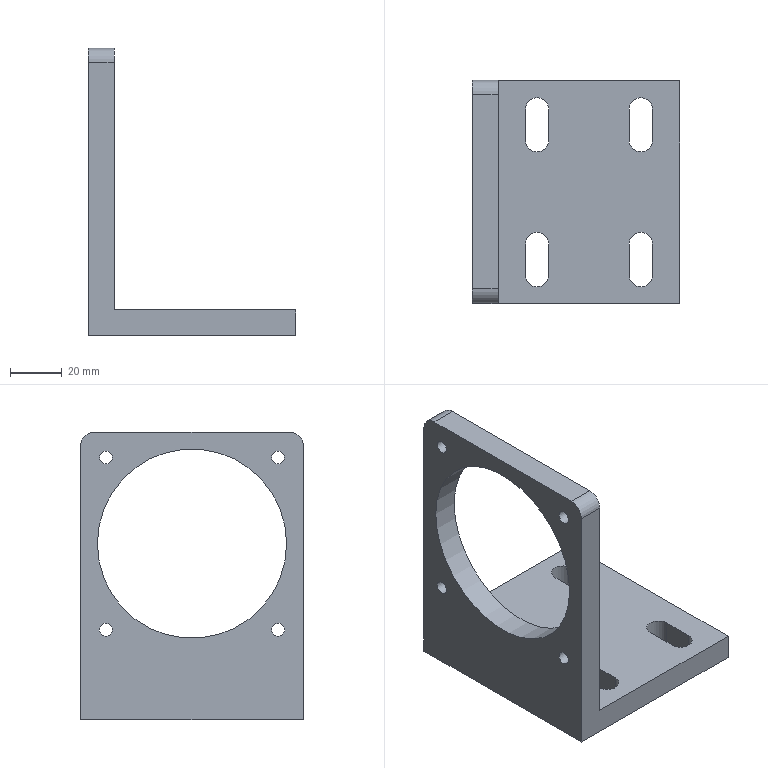Part | NX | features 5003_219_Bracket 2 | 1 solid | 31 faces | box 80 x 86 x 111 mm | volume 106026 mm3 | plane 16 | cylinder 15 | commonest cylinder face diameters 9 x8 5 x4 11 x2 73 x1
STEP:
#1=CARTESIAN_POINT('',(-21.725,90.734,-85.766));
#2=VERTEX_POINT('',#1);
#3=CARTESIAN_POINT('',(-21.725,88.234,-85.766));
#4=DIRECTION('',(-1.,0.,0.));
#5=DIRECTION('',(0.,1.,0.));
#6=AXIS2_PLACEMENT_3D('',#3,#4,#5);
#7=CIRCLE('',#6,2.5);
#8=EDGE_CURVE('',#2,#2,#7,.T.);
#9=ORIENTED_EDGE('',*,*,#8,.F.);
#10=EDGE_LOOP('',(#9));
#11=FACE_BOUND('',#10,.T.);
#12=CARTESIAN_POINT('',(-21.725,90.734,-152.234));
#13=VERTEX_POINT('',#12);
#14=CARTESIAN_POINT('',(-21.725,88.234,-152.234));
#15=DIRECTION('',(-1.,0.,0.));
#16=DIRECTION('',(0.,1.,0.));
#17=AXIS2_PLACEMENT_3D('',#14,#15,#16);
#18=CIRCLE('',#17,2.5);
#19=EDGE_CURVE('',#13,#13,#18,.T.);
#20=ORIENTED_EDGE('',*,*,#19,.F.);
#21=EDGE_LOOP('',(#20));
#22=FACE_BOUND('',#21,.T.);
#23=CARTESIAN_POINT('',(-21.725,24.266,-152.234));
#24=VERTEX_POINT('',#23);
#25=CARTESIAN_POINT('',(-21.725,21.766,-152.234));
#26=DIRECTION('',(-1.,0.,0.));
#27=DIRECTION('',(0.,1.,0.));
#28=AXIS2_PLACEMENT_3D('',#25,#26,#27);
#29=CIRCLE('',#28,2.5);
#30=EDGE_CURVE('',#24,#24,#29,.T.);
#31=ORIENTED_EDGE('',*,*,#30,.F.);
#32=EDGE_LOOP('',(#31));
#33=FACE_BOUND('',#32,.T.);
#34=CARTESIAN_POINT('',(-21.725,24.266,-85.766));
#35=VERTEX_POINT('',#34);
#36=CARTESIAN_POINT('',(-21.725,21.766,-85.766));
#37=DIRECTION('',(-1.,0.,0.));
#38=DIRECTION('',(0.,1.,0.));
#39=AXIS2_PLACEMENT_3D('',#36,#37,#38);
#40=CIRCLE('',#39,2.5);
#41=EDGE_CURVE('',#35,#35,#40,.T.);
#42=ORIENTED_EDGE('',*,*,#41,.F.);
#43=EDGE_LOOP('',(#42));
#44=FACE_BOUND('',#43,.T.);
#45=CARTESIAN_POINT('',(-21.725,91.5,-119.));
#46=VERTEX_POINT('',#45);
#47=CARTESIAN_POINT('',(-21.725,55.,-119.));
#48=DIRECTION('',(-1.,0.,0.));
#49=DIRECTION('',(0.,1.,0.));
#50=AXIS2_PLACEMENT_3D('',#47,#48,#49);
#51=CIRCLE('',#50,36.5);
#52=EDGE_CURVE('',#46,#46,#51,.T.);
#53=ORIENTED_EDGE('',*,*,#52,.F.);
#54=EDGE_LOOP('',(#53));
#55=FACE_BOUND('',#54,.T.);
#56=CARTESIAN_POINT('',(-21.725,12.,-187.));
#57=VERTEX_POINT('',#56);
#58=CARTESIAN_POINT('',(-21.725,12.,-81.5));
#59=VERTEX_POINT('',#58);
#60=CARTESIAN_POINT('',(-21.725,12.,-187.));
#61=DIRECTION('',(0.,0.,1.));
#62=VECTOR('',#61,1000.);
#63=LINE('',#60,#62);
#64=EDGE_CURVE('',#57,#59,#63,.T.);
#65=ORIENTED_EDGE('',*,*,#64,.T.);
#66=CARTESIAN_POINT('',(-21.725,17.5,-76.));
#67=VERTEX_POINT('',#66);
#68=CARTESIAN_POINT('',(-21.725,17.5,-81.5));
#69=DIRECTION('',(-1.,0.,0.));
#70=DIRECTION('',(0.,0.,1.));
#71=AXIS2_PLACEMENT_3D('',#68,#69,#70);
#72=CIRCLE('',#71,5.5);
#73=EDGE_CURVE('',#59,#67,#72,.T.);
#74=ORIENTED_EDGE('',*,*,#73,.T.);
#75=CARTESIAN_POINT('',(-21.725,92.5,-76.));
#76=VERTEX_POINT('',#75);
#77=CARTESIAN_POINT('',(-21.725,12.,-76.));
#78=DIRECTION('',(0.,1.,0.));
#79=VECTOR('',#78,1000.);
#80=LINE('',#77,#79);
#81=EDGE_CURVE('',#67,#76,#80,.T.);
#82=ORIENTED_EDGE('',*,*,#81,.T.);
#83=CARTESIAN_POINT('',(-21.725,98.,-81.5));
#84=VERTEX_POINT('',#83);
#85=CARTESIAN_POINT('',(-21.725,92.5,-81.5));
#86=DIRECTION('',(-1.,0.,0.));
#87=DIRECTION('',(0.,0.,1.));
#88=AXIS2_PLACEMENT_3D('',#85,#86,#87);
#89=CIRCLE('',#88,5.5);
#90=EDGE_CURVE('',#76,#84,#89,.T.);
#91=ORIENTED_EDGE('',*,*,#90,.T.);
#92=CARTESIAN_POINT('',(-21.725,98.,-187.));
#93=VERTEX_POINT('',#92);
#94=CARTESIAN_POINT('',(-21.725,98.,-187.));
#95=DIRECTION('',(0.,0.,1.));
#96=VECTOR('',#95,1000.);
#97=LINE('',#94,#96);
#98=EDGE_CURVE('',#93,#84,#97,.T.);
#99=ORIENTED_EDGE('',*,*,#98,.F.);
#100=CARTESIAN_POINT('',(-21.725,12.,-187.));
#101=DIRECTION('',(0.,1.,0.));
#102=VECTOR('',#101,1000.);
#103=LINE('',#100,#102);
#104=EDGE_CURVE('',#57,#93,#103,.T.);
#105=ORIENTED_EDGE('',*,*,#104,.F.);
#106=EDGE_LOOP('',(#65,#74,#82,#91,#99,#105));
#107=FACE_BOUND('',#106,.T.);
#108=CARTESIAN_POINT('',(-21.725,12.,-187.));
#109=DIRECTION('',(-1.,0.,0.));
#110=DIRECTION('',(0.,0.,1.));
#111=AXIS2_PLACEMENT_3D('',#108,#109,#110);
#112=PLANE('',#111);
#113=ADVANCED_FACE('',(#11,#22,#33,#44,#55,#107),#112,.T.);
#114=CARTESIAN_POINT('',(38.775,23.,-187.));
#115=VERTEX_POINT('',#114);
#116=CARTESIAN_POINT('',(47.775,23.,-187.));
#117=VERTEX_POINT('',#116);
#118=CARTESIAN_POINT('',(43.275,23.,-187.));
#119=DIRECTION('',(0.,0.,-1.));
#120=DIRECTION('',(-1.,0.,0.));
#121=AXIS2_PLACEMENT_3D('',#118,#119,#120);
#122=CIRCLE('',#121,4.5);
#123=EDGE_CURVE('',#115,#117,#122,.F.);
#124=ORIENTED_EDGE('',*,*,#123,.T.);
#125=CARTESIAN_POINT('',(47.775,35.,-187.));
#126=VERTEX_POINT('',#125);
#127=CARTESIAN_POINT('',(47.775,23.,-187.));
#128=DIRECTION('',(0.,1.,0.));
#129=VECTOR('',#128,1000.);
#130=LINE('',#127,#129);
#131=EDGE_CURVE('',#117,#126,#130,.T.);
#132=ORIENTED_EDGE('',*,*,#131,.T.);
#133=CARTESIAN_POINT('',(38.775,35.,-187.));
#134=VERTEX_POINT('',#133);
#135=CARTESIAN_POINT('',(43.275,35.,-187.));
#136=DIRECTION('',(0.,0.,-1.));
#137=DIRECTION('',(-1.,0.,0.));
#138=AXIS2_PLACEMENT_3D('',#135,#136,#137);
#139=CIRCLE('',#138,4.5);
#140=EDGE_CURVE('',#126,#134,#139,.F.);
#141=ORIENTED_EDGE('',*,*,#140,.T.);
#142=CARTESIAN_POINT('',(38.775,23.,-187.));
#143=DIRECTION('',(0.,-1.,0.));
#144=VECTOR('',#143,1000.);
#145=LINE('',#142,#144);
#146=EDGE_CURVE('',#134,#115,#145,.T.);
#147=ORIENTED_EDGE('',*,*,#146,.T.);
#148=EDGE_LOOP('',(#124,#132,#141,#147));
#149=FACE_BOUND('',#148,.T.);
#150=CARTESIAN_POINT('',(38.775,75.,-187.));
#151=VERTEX_POINT('',#150);
#152=CARTESIAN_POINT('',(47.775,75.,-187.));
#153=VERTEX_POINT('',#152);
#154=CARTESIAN_POINT('',(43.275,75.,-187.));
#155=DIRECTION('',(0.,0.,-1.));
#156=DIRECTION('',(-1.,0.,0.));
#157=AXIS2_PLACEMENT_3D('',#154,#155,#156);
#158=CIRCLE('',#157,4.5);
#159=EDGE_CURVE('',#151,#153,#158,.F.);
#160=ORIENTED_EDGE('',*,*,#159,.T.);
#161=CARTESIAN_POINT('',(47.775,87.,-187.));
#162=VERTEX_POINT('',#161);
#163=CARTESIAN_POINT('',(47.775,75.,-187.));
#164=DIRECTION('',(0.,1.,0.));
#165=VECTOR('',#164,1000.);
#166=LINE('',#163,#165);
#167=EDGE_CURVE('',#153,#162,#166,.T.);
#168=ORIENTED_EDGE('',*,*,#167,.T.);
#169=CARTESIAN_POINT('',(38.775,87.,-187.));
#170=VERTEX_POINT('',#169);
#171=CARTESIAN_POINT('',(43.275,87.,-187.));
#172=DIRECTION('',(0.,0.,-1.));
#173=DIRECTION('',(-1.,0.,0.));
#174=AXIS2_PLACEMENT_3D('',#171,#172,#173);
#175=CIRCLE('',#174,4.5);
#176=EDGE_CURVE('',#162,#170,#175,.F.);
#177=ORIENTED_EDGE('',*,*,#176,.T.);
#178=CARTESIAN_POINT('',(38.775,75.,-187.));
#179=DIRECTION('',(0.,-1.,0.));
#180=VECTOR('',#179,1000.);
#181=LINE('',#178,#180);
#182=EDGE_CURVE('',#170,#151,#181,.T.);
#183=ORIENTED_EDGE('',*,*,#182,.T.);
#184=EDGE_LOOP('',(#160,#168,#177,#183));
#185=FACE_BOUND('',#184,.T.);
#186=CARTESIAN_POINT('',(-1.225,75.,-187.));
#187=VERTEX_POINT('',#186);
#188=CARTESIAN_POINT('',(7.775,75.,-187.));
#189=VERTEX_POINT('',#188);
#190=CARTESIAN_POINT('',(3.275,75.,-187.));
#191=DIRECTION('',(0.,0.,-1.));
#192=DIRECTION('',(-1.,0.,0.));
#193=AXIS2_PLACEMENT_3D('',#190,#191,#192);
#194=CIRCLE('',#193,4.5);
#195=EDGE_CURVE('',#187,#189,#194,.F.);
#196=ORIENTED_EDGE('',*,*,#195,.T.);
#197=CARTESIAN_POINT('',(7.775,87.,-187.));
#198=VERTEX_POINT('',#197);
#199=CARTESIAN_POINT('',(7.775,75.,-187.));
#200=DIRECTION('',(0.,1.,0.));
#201=VECTOR('',#200,1000.);
#202=LINE('',#199,#201);
#203=EDGE_CURVE('',#189,#198,#202,.T.);
#204=ORIENTED_EDGE('',*,*,#203,.T.);
#205=CARTESIAN_POINT('',(-1.225,87.,-187.));
#206=VERTEX_POINT('',#205);
#207=CARTESIAN_POINT('',(3.275,87.,-187.));
#208=DIRECTION('',(0.,0.,-1.));
#209=DIRECTION('',(-1.,0.,0.));
#210=AXIS2_PLACEMENT_3D('',#207,#208,#209);
#211=CIRCLE('',#210,4.5);
#212=EDGE_CURVE('',#198,#206,#211,.F.);
#213=ORIENTED_EDGE('',*,*,#212,.T.);
#214=CARTESIAN_POINT('',(-1.225,75.,-187.));
#215=DIRECTION('',(0.,-1.,0.));
#216=VECTOR('',#215,1000.);
#217=LINE('',#214,#216);
#218=EDGE_CURVE('',#206,#187,#217,.T.);
#219=ORIENTED_EDGE('',*,*,#218,.T.);
#220=EDGE_LOOP('',(#196,#204,#213,#219));
#221=FACE_BOUND('',#220,.T.);
#222=CARTESIAN_POINT('',(-1.225,23.,-187.));
#223=VERTEX_POINT('',#222);
#224=CARTESIAN_POINT('',(7.775,23.,-187.));
#225=VERTEX_POINT('',#224);
#226=CARTESIAN_POINT('',(3.275,23.,-187.));
#227=DIRECTION('',(0.,0.,-1.));
#228=DIRECTION('',(-1.,0.,0.));
#229=AXIS2_PLACEMENT_3D('',#226,#227,#228);
#230=CIRCLE('',#229,4.5);
#231=EDGE_CURVE('',#223,#225,#230,.F.);
#232=ORIENTED_EDGE('',*,*,#231,.T.);
#233=CARTESIAN_POINT('',(7.775,35.,-187.));
#234=VERTEX_POINT('',#233);
#235=CARTESIAN_POINT('',(7.775,23.,-187.));
#236=DIRECTION('',(0.,1.,0.));
#237=VECTOR('',#236,1000.);
#238=LINE('',#235,#237);
#239=EDGE_CURVE('',#225,#234,#238,.T.);
#240=ORIENTED_EDGE('',*,*,#239,.T.);
#241=CARTESIAN_POINT('',(-1.225,35.,-187.));
#242=VERTEX_POINT('',#241);
#243=CARTESIAN_POINT('',(3.275,35.,-187.));
#244=DIRECTION('',(0.,0.,-1.));
#245=DIRECTION('',(-1.,0.,0.));
#246=AXIS2_PLACEMENT_3D('',#243,#244,#245);
#247=CIRCLE('',#246,4.5);
#248=EDGE_CURVE('',#234,#242,#247,.F.);
#249=ORIENTED_EDGE('',*,*,#248,.T.);
#250=CARTESIAN_POINT('',(-1.225,23.,-187.));
#251=DIRECTION('',(0.,-1.,0.));
#252=VECTOR('',#251,1000.);
#253=LINE('',#250,#252);
#254=EDGE_CURVE('',#242,#223,#253,.T.);
#255=ORIENTED_EDGE('',*,*,#254,.T.);
#256=EDGE_LOOP('',(#232,#240,#249,#255));
#257=FACE_BOUND('',#256,.T.);
#258=ORIENTED_EDGE('',*,*,#104,.T.);
#259=CARTESIAN_POINT('',(58.275,98.,-187.));
#260=VERTEX_POINT('',#259);
#261=CARTESIAN_POINT('',(-21.725,98.,-187.));
#262=DIRECTION('',(-1.,0.,0.));
#263=VECTOR('',#262,1000.);
#264=LINE('',#261,#263);
#265=EDGE_CURVE('',#260,#93,#264,.T.);
#266=ORIENTED_EDGE('',*,*,#265,.F.);
#267=CARTESIAN_POINT('',(58.275,12.,-187.));
#268=VERTEX_POINT('',#267);
#269=CARTESIAN_POINT('',(58.275,12.,-187.));
#270=DIRECTION('',(0.,1.,0.));
#271=VECTOR('',#270,1000.);
#272=LINE('',#269,#271);
#273=EDGE_CURVE('',#268,#260,#272,.T.);
#274=ORIENTED_EDGE('',*,*,#273,.F.);
#275=CARTESIAN_POINT('',(-21.725,12.,-187.));
#276=DIRECTION('',(-1.,0.,0.));
#277=VECTOR('',#276,1000.);
#278=LINE('',#275,#277);
#279=EDGE_CURVE('',#268,#57,#278,.T.);
#280=ORIENTED_EDGE('',*,*,#279,.T.);
#281=EDGE_LOOP('',(#258,#266,#274,#280));
#282=FACE_BOUND('',#281,.T.);
#283=CARTESIAN_POINT('',(-21.725,12.,-187.));
#284=DIRECTION('',(0.,0.,-1.));
#285=DIRECTION('',(-1.,0.,0.));
#286=AXIS2_PLACEMENT_3D('',#283,#284,#285);
#287=PLANE('',#286);
#288=ADVANCED_FACE('',(#149,#185,#221,#257,#282),#287,.T.);
#289=ORIENTED_EDGE('',*,*,#273,.T.);
#290=CARTESIAN_POINT('',(58.275,98.,-177.));
#291=VERTEX_POINT('',#290);
#292=CARTESIAN_POINT('',(58.275,98.,-187.));
#293=DIRECTION('',(0.,0.,-1.));
#294=VECTOR('',#293,1000.);
#295=LINE('',#292,#294);
#296=EDGE_CURVE('',#291,#260,#295,.T.);
#297=ORIENTED_EDGE('',*,*,#296,.F.);
#298=CARTESIAN_POINT('',(58.275,12.,-177.));
#299=VERTEX_POINT('',#298);
#300=CARTESIAN_POINT('',(58.275,12.,-177.));
#301=DIRECTION('',(0.,1.,0.));
#302=VECTOR('',#301,1000.);
#303=LINE('',#300,#302);
#304=EDGE_CURVE('',#299,#291,#303,.T.);
#305=ORIENTED_EDGE('',*,*,#304,.F.);
#306=CARTESIAN_POINT('',(58.275,12.,-187.));
#307=DIRECTION('',(0.,0.,-1.));
#308=VECTOR('',#307,1000.);
#309=LINE('',#306,#308);
#310=EDGE_CURVE('',#299,#268,#309,.T.);
#311=ORIENTED_EDGE('',*,*,#310,.T.);
#312=EDGE_LOOP('',(#289,#297,#305,#311));
#313=FACE_BOUND('',#312,.T.);
#314=CARTESIAN_POINT('',(58.275,12.,-187.));
#315=DIRECTION('',(1.,0.,0.));
#316=DIRECTION('',(0.,-1.,0.));
#317=AXIS2_PLACEMENT_3D('',#314,#315,#316);
#318=PLANE('',#317);
#319=ADVANCED_FACE('',(#313),#318,.T.);
#320=CARTESIAN_POINT('',(38.775,23.,-177.));
#321=VERTEX_POINT('',#320);
#322=CARTESIAN_POINT('',(47.775,23.,-177.));
#323=VERTEX_POINT('',#322);
#324=CARTESIAN_POINT('',(43.275,23.,-177.));
#325=DIRECTION('',(0.,0.,1.));
#326=DIRECTION('',(1.,0.,0.));
#327=AXIS2_PLACEMENT_3D('',#324,#325,#326);
#328=CIRCLE('',#327,4.5);
#329=EDGE_CURVE('',#321,#323,#328,.T.);
#330=ORIENTED_EDGE('',*,*,#329,.F.);
#331=CARTESIAN_POINT('',(38.775,35.,-177.));
#332=VERTEX_POINT('',#331);
#333=CARTESIAN_POINT('',(38.775,23.,-177.));
#334=DIRECTION('',(0.,-1.,0.));
#335=VECTOR('',#334,1000.);
#336=LINE('',#333,#335);
#337=EDGE_CURVE('',#332,#321,#336,.T.);
#338=ORIENTED_EDGE('',*,*,#337,.F.);
#339=CARTESIAN_POINT('',(47.775,35.,-177.));
#340=VERTEX_POINT('',#339);
#341=CARTESIAN_POINT('',(43.275,35.,-177.));
#342=DIRECTION('',(0.,0.,1.));
#343=DIRECTION('',(1.,0.,0.));
#344=AXIS2_PLACEMENT_3D('',#341,#342,#343);
#345=CIRCLE('',#344,4.5);
#346=EDGE_CURVE('',#340,#332,#345,.T.);
#347=ORIENTED_EDGE('',*,*,#346,.F.);
#348=CARTESIAN_POINT('',(47.775,23.,-177.));
#349=DIRECTION('',(0.,1.,0.));
#350=VECTOR('',#349,1000.);
#351=LINE('',#348,#350);
#352=EDGE_CURVE('',#323,#340,#351,.T.);
#353=ORIENTED_EDGE('',*,*,#352,.F.);
#354=EDGE_LOOP('',(#330,#338,#347,#353));
#355=FACE_BOUND('',#354,.T.);
#356=CARTESIAN_POINT('',(38.775,75.,-177.));
#357=VERTEX_POINT('',#356);
#358=CARTESIAN_POINT('',(47.775,75.,-177.));
#359=VERTEX_POINT('',#358);
#360=CARTESIAN_POINT('',(43.275,75.,-177.));
#361=DIRECTION('',(0.,0.,1.));
#362=DIRECTION('',(1.,0.,0.));
#363=AXIS2_PLACEMENT_3D('',#360,#361,#362);
#364=CIRCLE('',#363,4.5);
#365=EDGE_CURVE('',#357,#359,#364,.T.);
#366=ORIENTED_EDGE('',*,*,#365,.F.);
#367=CARTESIAN_POINT('',(38.775,87.,-177.));
#368=VERTEX_POINT('',#367);
#369=CARTESIAN_POINT('',(38.775,75.,-177.));
#370=DIRECTION('',(0.,-1.,0.));
#371=VECTOR('',#370,1000.);
#372=LINE('',#369,#371);
#373=EDGE_CURVE('',#368,#357,#372,.T.);
#374=ORIENTED_EDGE('',*,*,#373,.F.);
#375=CARTESIAN_POINT('',(47.775,87.,-177.));
#376=VERTEX_POINT('',#375);
#377=CARTESIAN_POINT('',(43.275,87.,-177.));
#378=DIRECTION('',(0.,0.,1.));
#379=DIRECTION('',(1.,0.,0.));
#380=AXIS2_PLACEMENT_3D('',#377,#378,#379);
#381=CIRCLE('',#380,4.5);
#382=EDGE_CURVE('',#376,#368,#381,.T.);
#383=ORIENTED_EDGE('',*,*,#382,.F.);
#384=CARTESIAN_POINT('',(47.775,75.,-177.));
#385=DIRECTION('',(0.,1.,0.));
#386=VECTOR('',#385,1000.);
#387=LINE('',#384,#386);
#388=EDGE_CURVE('',#359,#376,#387,.T.);
#389=ORIENTED_EDGE('',*,*,#388,.F.);
#390=EDGE_LOOP('',(#366,#374,#383,#389));
#391=FACE_BOUND('',#390,.T.);
#392=CARTESIAN_POINT('',(-1.225,75.,-177.));
#393=VERTEX_POINT('',#392);
#394=CARTESIAN_POINT('',(7.775,75.,-177.));
#395=VERTEX_POINT('',#394);
#396=CARTESIAN_POINT('',(3.275,75.,-177.));
#397=DIRECTION('',(0.,0.,1.));
#398=DIRECTION('',(1.,0.,0.));
#399=AXIS2_PLACEMENT_3D('',#396,#397,#398);
#400=CIRCLE('',#399,4.5);
#401=EDGE_CURVE('',#393,#395,#400,.T.);
#402=ORIENTED_EDGE('',*,*,#401,.F.);
#403=CARTESIAN_POINT('',(-1.225,87.,-177.));
#404=VERTEX_POINT('',#403);
#405=CARTESIAN_POINT('',(-1.225,75.,-177.));
#406=DIRECTION('',(0.,-1.,0.));
#407=VECTOR('',#406,1000.);
#408=LINE('',#405,#407);
#409=EDGE_CURVE('',#404,#393,#408,.T.);
#410=ORIENTED_EDGE('',*,*,#409,.F.);
#411=CARTESIAN_POINT('',(7.775,87.,-177.));
#412=VERTEX_POINT('',#411);
#413=CARTESIAN_POINT('',(3.275,87.,-177.));
#414=DIRECTION('',(0.,0.,1.));
#415=DIRECTION('',(1.,0.,0.));
#416=AXIS2_PLACEMENT_3D('',#413,#414,#415);
#417=CIRCLE('',#416,4.5);
#418=EDGE_CURVE('',#412,#404,#417,.T.);
#419=ORIENTED_EDGE('',*,*,#418,.F.);
#420=CARTESIAN_POINT('',(7.775,75.,-177.));
#421=DIRECTION('',(0.,1.,0.));
#422=VECTOR('',#421,1000.);
#423=LINE('',#420,#422);
#424=EDGE_CURVE('',#395,#412,#423,.T.);
#425=ORIENTED_EDGE('',*,*,#424,.F.);
#426=EDGE_LOOP('',(#402,#410,#419,#425));
#427=FACE_BOUND('',#426,.T.);
#428=CARTESIAN_POINT('',(-1.225,23.,-177.));
#429=VERTEX_POINT('',#428);
#430=CARTESIAN_POINT('',(7.775,23.,-177.));
#431=VERTEX_POINT('',#430);
#432=CARTESIAN_POINT('',(3.275,23.,-177.));
#433=DIRECTION('',(0.,0.,1.));
#434=DIRECTION('',(1.,0.,0.));
#435=AXIS2_PLACEMENT_3D('',#432,#433,#434);
#436=CIRCLE('',#435,4.5);
#437=EDGE_CURVE('',#429,#431,#436,.T.);
#438=ORIENTED_EDGE('',*,*,#437,.F.);
#439=CARTESIAN_POINT('',(-1.225,35.,-177.));
#440=VERTEX_POINT('',#439);
#441=CARTESIAN_POINT('',(-1.225,23.,-177.));
#442=DIRECTION('',(0.,-1.,0.));
#443=VECTOR('',#442,1000.);
#444=LINE('',#441,#443);
#445=EDGE_CURVE('',#440,#429,#444,.T.);
#446=ORIENTED_EDGE('',*,*,#445,.F.);
#447=CARTESIAN_POINT('',(7.775,35.,-177.));
#448=VERTEX_POINT('',#447);
#449=CARTESIAN_POINT('',(3.275,35.,-177.));
#450=DIRECTION('',(0.,0.,1.));
#451=DIRECTION('',(1.,0.,0.));
#452=AXIS2_PLACEMENT_3D('',#449,#450,#451);
#453=CIRCLE('',#452,4.5);
#454=EDGE_CURVE('',#448,#440,#453,.T.);
#455=ORIENTED_EDGE('',*,*,#454,.F.);
#456=CARTESIAN_POINT('',(7.775,23.,-177.));
#457=DIRECTION('',(0.,1.,0.));
#458=VECTOR('',#457,1000.);
#459=LINE('',#456,#458);
#460=EDGE_CURVE('',#431,#448,#459,.T.);
#461=ORIENTED_EDGE('',*,*,#460,.F.);
#462=EDGE_LOOP('',(#438,#446,#455,#461));
#463=FACE_BOUND('',#462,.T.);
#464=ORIENTED_EDGE('',*,*,#304,.T.);
#465=CARTESIAN_POINT('',(-11.725,98.,-177.));
#466=VERTEX_POINT('',#465);
#467=CARTESIAN_POINT('',(-11.725,98.,-177.));
#468=DIRECTION('',(1.,0.,0.));
#469=VECTOR('',#468,1000.);
#470=LINE('',#467,#469);
#471=EDGE_CURVE('',#466,#291,#470,.T.);
#472=ORIENTED_EDGE('',*,*,#471,.F.);
#473=CARTESIAN_POINT('',(-11.725,12.,-177.));
#474=VERTEX_POINT('',#473);
#475=CARTESIAN_POINT('',(-11.725,12.,-177.));
#476=DIRECTION('',(0.,1.,0.));
#477=VECTOR('',#476,1000.);
#478=LINE('',#475,#477);
#479=EDGE_CURVE('',#474,#466,#478,.T.);
#480=ORIENTED_EDGE('',*,*,#479,.F.);
#481=CARTESIAN_POINT('',(-11.725,12.,-177.));
#482=DIRECTION('',(1.,0.,0.));
#483=VECTOR('',#482,1000.);
#484=LINE('',#481,#483);
#485=EDGE_CURVE('',#474,#299,#484,.T.);
#486=ORIENTED_EDGE('',*,*,#485,.T.);
#487=EDGE_LOOP('',(#464,#472,#480,#486));
#488=FACE_BOUND('',#487,.T.);
#489=CARTESIAN_POINT('',(-11.725,12.,-177.));
#490=DIRECTION('',(0.,0.,1.));
#491=DIRECTION('',(1.,0.,0.));
#492=AXIS2_PLACEMENT_3D('',#489,#490,#491);
#493=PLANE('',#492);
#494=ADVANCED_FACE('',(#355,#391,#427,#463,#488),#493,.T.);
#495=CARTESIAN_POINT('',(-11.725,85.734,-85.766));
#496=VERTEX_POINT('',#495);
#497=CARTESIAN_POINT('',(-11.725,88.234,-85.766));
#498=DIRECTION('',(1.,0.,0.));
#499=DIRECTION('',(0.,-1.,0.));
#500=AXIS2_PLACEMENT_3D('',#497,#498,#499);
#501=CIRCLE('',#500,2.5);
#502=EDGE_CURVE('',#496,#496,#501,.T.);
#503=ORIENTED_EDGE('',*,*,#502,.F.);
#504=EDGE_LOOP('',(#503));
#505=FACE_BOUND('',#504,.T.);
#506=CARTESIAN_POINT('',(-11.725,85.734,-152.234));
#507=VERTEX_POINT('',#506);
#508=CARTESIAN_POINT('',(-11.725,88.234,-152.234));
#509=DIRECTION('',(1.,0.,0.));
#510=DIRECTION('',(0.,-1.,0.));
#511=AXIS2_PLACEMENT_3D('',#508,#509,#510);
#512=CIRCLE('',#511,2.5);
#513=EDGE_CURVE('',#507,#507,#512,.T.);
#514=ORIENTED_EDGE('',*,*,#513,.F.);
#515=EDGE_LOOP('',(#514));
#516=FACE_BOUND('',#515,.T.);
#517=CARTESIAN_POINT('',(-11.725,19.266,-152.234));
#518=VERTEX_POINT('',#517);
#519=CARTESIAN_POINT('',(-11.725,21.766,-152.234));
#520=DIRECTION('',(1.,0.,0.));
#521=DIRECTION('',(0.,-1.,0.));
#522=AXIS2_PLACEMENT_3D('',#519,#520,#521);
#523=CIRCLE('',#522,2.5);
#524=EDGE_CURVE('',#518,#518,#523,.T.);
#525=ORIENTED_EDGE('',*,*,#524,.F.);
#526=EDGE_LOOP('',(#525));
#527=FACE_BOUND('',#526,.T.);
#528=CARTESIAN_POINT('',(-11.725,19.266,-85.766));
#529=VERTEX_POINT('',#528);
#530=CARTESIAN_POINT('',(-11.725,21.766,-85.766));
#531=DIRECTION('',(1.,0.,0.));
#532=DIRECTION('',(0.,-1.,0.));
#533=AXIS2_PLACEMENT_3D('',#530,#531,#532);
#534=CIRCLE('',#533,2.5);
#535=EDGE_CURVE('',#529,#529,#534,.T.);
#536=ORIENTED_EDGE('',*,*,#535,.F.);
#537=EDGE_LOOP('',(#536));
#538=FACE_BOUND('',#537,.T.);
#539=CARTESIAN_POINT('',(-11.725,18.5,-119.));
#540=VERTEX_POINT('',#539);
#541=CARTESIAN_POINT('',(-11.725,55.,-119.));
#542=DIRECTION('',(1.,0.,0.));
#543=DIRECTION('',(0.,-1.,0.));
#544=AXIS2_PLACEMENT_3D('',#541,#542,#543);
#545=CIRCLE('',#544,36.5);
#546=EDGE_CURVE('',#540,#540,#545,.F.);
#547=ORIENTED_EDGE('',*,*,#546,.T.);
#548=EDGE_LOOP('',(#547));
#549=FACE_BOUND('',#548,.T.);
#550=CARTESIAN_POINT('',(-11.725,17.5,-76.));
#551=VERTEX_POINT('',#550);
#552=CARTESIAN_POINT('',(-11.725,92.5,-76.));
#553=VERTEX_POINT('',#552);
#554=CARTESIAN_POINT('',(-11.725,12.,-76.));
#555=DIRECTION('',(0.,1.,0.));
#556=VECTOR('',#555,1000.);
#557=LINE('',#554,#556);
#558=EDGE_CURVE('',#551,#553,#557,.T.);
#559=ORIENTED_EDGE('',*,*,#558,.F.);
#560=CARTESIAN_POINT('',(-11.725,12.,-81.5));
#561=VERTEX_POINT('',#560);
#562=CARTESIAN_POINT('',(-11.725,17.5,-81.5));
#563=DIRECTION('',(1.,0.,0.));
#564=DIRECTION('',(0.,-1.,0.));
#565=AXIS2_PLACEMENT_3D('',#562,#563,#564);
#566=CIRCLE('',#565,5.5);
#567=EDGE_CURVE('',#551,#561,#566,.T.);
#568=ORIENTED_EDGE('',*,*,#567,.T.);
#569=CARTESIAN_POINT('',(-11.725,12.,-177.));
#570=DIRECTION('',(0.,0.,-1.));
#571=VECTOR('',#570,1000.);
#572=LINE('',#569,#571);
#573=EDGE_CURVE('',#561,#474,#572,.T.);
#574=ORIENTED_EDGE('',*,*,#573,.T.);
#575=ORIENTED_EDGE('',*,*,#479,.T.);
#576=CARTESIAN_POINT('',(-11.725,98.,-81.5));
#577=VERTEX_POINT('',#576);
#578=CARTESIAN_POINT('',(-11.725,98.,-177.));
#579=DIRECTION('',(0.,0.,-1.));
#580=VECTOR('',#579,1000.);
#581=LINE('',#578,#580);
#582=EDGE_CURVE('',#577,#466,#581,.T.);
#583=ORIENTED_EDGE('',*,*,#582,.F.);
#584=CARTESIAN_POINT('',(-11.725,92.5,-81.5));
#585=DIRECTION('',(1.,0.,0.));
#586=DIRECTION('',(0.,-1.,0.));
#587=AXIS2_PLACEMENT_3D('',#584,#585,#586);
#588=CIRCLE('',#587,5.5);
#589=EDGE_CURVE('',#577,#553,#588,.T.);
#590=ORIENTED_EDGE('',*,*,#589,.T.);
#591=EDGE_LOOP('',(#559,#568,#574,#575,#583,#590));
#592=FACE_BOUND('',#591,.T.);
#593=CARTESIAN_POINT('',(-11.725,12.,-177.));
#594=DIRECTION('',(1.,0.,0.));
#595=DIRECTION('',(0.,-1.,0.));
#596=AXIS2_PLACEMENT_3D('',#593,#594,#595);
#597=PLANE('',#596);
#598=ADVANCED_FACE('',(#505,#516,#527,#538,#549,#592),#597,.T.);
#599=ORIENTED_EDGE('',*,*,#81,.F.);
#600=CARTESIAN_POINT('',(-11.725,17.5,-76.));
#601=DIRECTION('',(1.,0.,0.));
#602=VECTOR('',#601,1000.);
#603=LINE('',#600,#602);
#604=EDGE_CURVE('',#67,#551,#603,.T.);
#605=ORIENTED_EDGE('',*,*,#604,.T.);
#606=ORIENTED_EDGE('',*,*,#558,.T.);
#607=CARTESIAN_POINT('',(-21.725,92.5,-76.));
#608=DIRECTION('',(1.,0.,0.));
#609=VECTOR('',#608,1000.);
#610=LINE('',#607,#609);
#611=EDGE_CURVE('',#553,#76,#610,.F.);
#612=ORIENTED_EDGE('',*,*,#611,.T.);
#613=EDGE_LOOP('',(#599,#605,#606,#612));
#614=FACE_BOUND('',#613,.T.);
#615=CARTESIAN_POINT('',(-21.725,12.,-76.));
#616=DIRECTION('',(0.,0.,1.));
#617=DIRECTION('',(1.,0.,0.));
#618=AXIS2_PLACEMENT_3D('',#615,#616,#617);
#619=PLANE('',#618);
#620=ADVANCED_FACE('',(#614),#619,.T.);
#621=ORIENTED_EDGE('',*,*,#573,.F.);
#622=CARTESIAN_POINT('',(-21.725,12.,-81.5));
#623=DIRECTION('',(1.,0.,0.));
#624=VECTOR('',#623,1000.);
#625=LINE('',#622,#624);
#626=EDGE_CURVE('',#561,#59,#625,.F.);
#627=ORIENTED_EDGE('',*,*,#626,.T.);
#628=ORIENTED_EDGE('',*,*,#64,.F.);
#629=ORIENTED_EDGE('',*,*,#279,.F.);
#630=ORIENTED_EDGE('',*,*,#310,.F.);
#631=ORIENTED_EDGE('',*,*,#485,.F.);
#632=EDGE_LOOP('',(#621,#627,#628,#629,#630,#631));
#633=FACE_BOUND('',#632,.T.);
#634=CARTESIAN_POINT('',(-21.725,12.,-187.));
#635=DIRECTION('',(0.,1.,0.));
#636=DIRECTION('',(1.,0.,0.));
#637=AXIS2_PLACEMENT_3D('',#634,#635,#636);
#638=PLANE('',#637);
#639=ADVANCED_FACE('',(#633),#638,.F.);
#640=ORIENTED_EDGE('',*,*,#98,.T.);
#641=CARTESIAN_POINT('',(-21.725,98.,-81.5));
#642=DIRECTION('',(1.,0.,0.));
#643=VECTOR('',#642,1000.);
#644=LINE('',#641,#643);
#645=EDGE_CURVE('',#84,#577,#644,.T.);
#646=ORIENTED_EDGE('',*,*,#645,.T.);
#647=ORIENTED_EDGE('',*,*,#582,.T.);
#648=ORIENTED_EDGE('',*,*,#471,.T.);
#649=ORIENTED_EDGE('',*,*,#296,.T.);
#650=ORIENTED_EDGE('',*,*,#265,.T.);
#651=EDGE_LOOP('',(#640,#646,#647,#648,#649,#650));
#652=FACE_BOUND('',#651,.T.);
#653=CARTESIAN_POINT('',(-21.725,98.,-187.));
#654=DIRECTION('',(0.,1.,0.));
#655=DIRECTION('',(1.,0.,0.));
#656=AXIS2_PLACEMENT_3D('',#653,#654,#655);
#657=PLANE('',#656);
#658=ADVANCED_FACE('',(#652),#657,.T.);
#659=ORIENTED_EDGE('',*,*,#546,.F.);
#660=EDGE_LOOP('',(#659));
#661=FACE_BOUND('',#660,.T.);
#662=ORIENTED_EDGE('',*,*,#52,.T.);
#663=EDGE_LOOP('',(#662));
#664=FACE_BOUND('',#663,.T.);
#665=CARTESIAN_POINT('',(58.276,55.,-119.));
#666=DIRECTION('',(-1.,0.,0.));
#667=DIRECTION('',(0.,1.,0.));
#668=AXIS2_PLACEMENT_3D('',#665,#666,#667);
#669=CYLINDRICAL_SURFACE('',#668,36.5);
#670=ADVANCED_FACE('',(#661,#664),#669,.F.);
#671=CARTESIAN_POINT('',(-1.225,23.,-187.001));
#672=DIRECTION('',(0.,0.,1.));
#673=VECTOR('',#672,1000.);
#674=LINE('',#671,#673);
#675=EDGE_CURVE('',#223,#429,#674,.T.);
#676=ORIENTED_EDGE('',*,*,#675,.T.);
#677=ORIENTED_EDGE('',*,*,#437,.T.);
#678=CARTESIAN_POINT('',(7.775,23.,-187.001));
#679=DIRECTION('',(0.,0.,1.));
#680=VECTOR('',#679,1000.);
#681=LINE('',#678,#680);
#682=EDGE_CURVE('',#225,#431,#681,.T.);
#683=ORIENTED_EDGE('',*,*,#682,.F.);
#684=ORIENTED_EDGE('',*,*,#231,.F.);
#685=EDGE_LOOP('',(#676,#677,#683,#684));
#686=FACE_BOUND('',#685,.T.);
#687=CARTESIAN_POINT('',(3.275,23.,-187.001));
#688=DIRECTION('',(0.,0.,1.));
#689=DIRECTION('',(1.,0.,0.));
#690=AXIS2_PLACEMENT_3D('',#687,#688,#689);
#691=CYLINDRICAL_SURFACE('',#690,4.5);
#692=ADVANCED_FACE('',(#686),#691,.F.);
#693=CARTESIAN_POINT('',(-1.225,35.,-187.001));
#694=DIRECTION('',(0.,0.,1.));
#695=VECTOR('',#694,1000.);
#696=LINE('',#693,#695);
#697=EDGE_CURVE('',#242,#440,#696,.T.);
#698=ORIENTED_EDGE('',*,*,#697,.T.);
#699=ORIENTED_EDGE('',*,*,#445,.T.);
#700=ORIENTED_EDGE('',*,*,#675,.F.);
#701=ORIENTED_EDGE('',*,*,#254,.F.);
#702=EDGE_LOOP('',(#698,#699,#700,#701));
#703=FACE_BOUND('',#702,.T.);
#704=CARTESIAN_POINT('',(-1.225,23.,-187.001));
#705=DIRECTION('',(-1.,0.,0.));
#706=DIRECTION('',(0.,1.,0.));
#707=AXIS2_PLACEMENT_3D('',#704,#705,#706);
#708=PLANE('',#707);
#709=ADVANCED_FACE('',(#703),#708,.F.);
#710=CARTESIAN_POINT('',(7.775,35.,-187.001));
#711=DIRECTION('',(0.,0.,1.));
#712=VECTOR('',#711,1000.);
#713=LINE('',#710,#712);
#714=EDGE_CURVE('',#234,#448,#713,.T.);
#715=ORIENTED_EDGE('',*,*,#714,.T.);
#716=ORIENTED_EDGE('',*,*,#454,.T.);
#717=ORIENTED_EDGE('',*,*,#697,.F.);
#718=ORIENTED_EDGE('',*,*,#248,.F.);
#719=EDGE_LOOP('',(#715,#716,#717,#718));
#720=FACE_BOUND('',#719,.T.);
#721=CARTESIAN_POINT('',(3.275,35.,-187.001));
#722=DIRECTION('',(0.,0.,1.));
#723=DIRECTION('',(1.,0.,0.));
#724=AXIS2_PLACEMENT_3D('',#721,#722,#723);
#725=CYLINDRICAL_SURFACE('',#724,4.5);
#726=ADVANCED_FACE('',(#720),#725,.F.);
#727=ORIENTED_EDGE('',*,*,#682,.T.);
#728=ORIENTED_EDGE('',*,*,#460,.T.);
#729=ORIENTED_EDGE('',*,*,#714,.F.);
#730=ORIENTED_EDGE('',*,*,#239,.F.);
#731=EDGE_LOOP('',(#727,#728,#729,#730));
#732=FACE_BOUND('',#731,.T.);
#733=CARTESIAN_POINT('',(7.775,23.,-187.001));
#734=DIRECTION('',(1.,0.,0.));
#735=DIRECTION('',(0.,-1.,0.));
#736=AXIS2_PLACEMENT_3D('',#733,#734,#735);
#737=PLANE('',#736);
#738=ADVANCED_FACE('',(#732),#737,.F.);
#739=CARTESIAN_POINT('',(-1.225,75.,-187.001));
#740=DIRECTION('',(0.,0.,1.));
#741=VECTOR('',#740,1000.);
#742=LINE('',#739,#741);
#743=EDGE_CURVE('',#187,#393,#742,.T.);
#744=ORIENTED_EDGE('',*,*,#743,.T.);
#745=ORIENTED_EDGE('',*,*,#401,.T.);
#746=CARTESIAN_POINT('',(7.775,75.,-187.001));
#747=DIRECTION('',(0.,0.,1.));
#748=VECTOR('',#747,1000.);
#749=LINE('',#746,#748);
#750=EDGE_CURVE('',#189,#395,#749,.T.);
#751=ORIENTED_EDGE('',*,*,#750,.F.);
#752=ORIENTED_EDGE('',*,*,#195,.F.);
#753=EDGE_LOOP('',(#744,#745,#751,#752));
#754=FACE_BOUND('',#753,.T.);
#755=CARTESIAN_POINT('',(3.275,75.,-187.001));
#756=DIRECTION('',(0.,0.,1.));
#757=DIRECTION('',(1.,0.,0.));
#758=AXIS2_PLACEMENT_3D('',#755,#756,#757);
#759=CYLINDRICAL_SURFACE('',#758,4.5);
#760=ADVANCED_FACE('',(#754),#759,.F.);
#761=CARTESIAN_POINT('',(-1.225,87.,-187.001));
#762=DIRECTION('',(0.,0.,1.));
#763=VECTOR('',#762,1000.);
#764=LINE('',#761,#763);
#765=EDGE_CURVE('',#206,#404,#764,.T.);
#766=ORIENTED_EDGE('',*,*,#765,.T.);
#767=ORIENTED_EDGE('',*,*,#409,.T.);
#768=ORIENTED_EDGE('',*,*,#743,.F.);
#769=ORIENTED_EDGE('',*,*,#218,.F.);
#770=EDGE_LOOP('',(#766,#767,#768,#769));
#771=FACE_BOUND('',#770,.T.);
#772=CARTESIAN_POINT('',(-1.225,75.,-187.001));
#773=DIRECTION('',(-1.,0.,0.));
#774=DIRECTION('',(0.,1.,0.));
#775=AXIS2_PLACEMENT_3D('',#772,#773,#774);
#776=PLANE('',#775);
#777=ADVANCED_FACE('',(#771),#776,.F.);
#778=CARTESIAN_POINT('',(7.775,87.,-187.001));
#779=DIRECTION('',(0.,0.,1.));
#780=VECTOR('',#779,1000.);
#781=LINE('',#778,#780);
#782=EDGE_CURVE('',#198,#412,#781,.T.);
#783=ORIENTED_EDGE('',*,*,#782,.T.);
#784=ORIENTED_EDGE('',*,*,#418,.T.);
#785=ORIENTED_EDGE('',*,*,#765,.F.);
#786=ORIENTED_EDGE('',*,*,#212,.F.);
#787=EDGE_LOOP('',(#783,#784,#785,#786));
#788=FACE_BOUND('',#787,.T.);
#789=CARTESIAN_POINT('',(3.275,87.,-187.001));
#790=DIRECTION('',(0.,0.,1.));
#791=DIRECTION('',(1.,0.,0.));
#792=AXIS2_PLACEMENT_3D('',#789,#790,#791);
#793=CYLINDRICAL_SURFACE('',#792,4.5);
#794=ADVANCED_FACE('',(#788),#793,.F.);
#795=ORIENTED_EDGE('',*,*,#750,.T.);
#796=ORIENTED_EDGE('',*,*,#424,.T.);
#797=ORIENTED_EDGE('',*,*,#782,.F.);
#798=ORIENTED_EDGE('',*,*,#203,.F.);
#799=EDGE_LOOP('',(#795,#796,#797,#798));
#800=FACE_BOUND('',#799,.T.);
#801=CARTESIAN_POINT('',(7.775,75.,-187.001));
#802=DIRECTION('',(1.,0.,0.));
#803=DIRECTION('',(0.,-1.,0.));
#804=AXIS2_PLACEMENT_3D('',#801,#802,#803);
#805=PLANE('',#804);
#806=ADVANCED_FACE('',(#800),#805,.F.);
#807=CARTESIAN_POINT('',(38.775,75.,-187.001));
#808=DIRECTION('',(0.,0.,1.));
#809=VECTOR('',#808,1000.);
#810=LINE('',#807,#809);
#811=EDGE_CURVE('',#151,#357,#810,.T.);
#812=ORIENTED_EDGE('',*,*,#811,.T.);
#813=ORIENTED_EDGE('',*,*,#365,.T.);
#814=CARTESIAN_POINT('',(47.775,75.,-187.001));
#815=DIRECTION('',(0.,0.,1.));
#816=VECTOR('',#815,1000.);
#817=LINE('',#814,#816);
#818=EDGE_CURVE('',#153,#359,#817,.T.);
#819=ORIENTED_EDGE('',*,*,#818,.F.);
#820=ORIENTED_EDGE('',*,*,#159,.F.);
#821=EDGE_LOOP('',(#812,#813,#819,#820));
#822=FACE_BOUND('',#821,.T.);
#823=CARTESIAN_POINT('',(43.275,75.,-187.001));
#824=DIRECTION('',(0.,0.,1.));
#825=DIRECTION('',(1.,0.,0.));
#826=AXIS2_PLACEMENT_3D('',#823,#824,#825);
#827=CYLINDRICAL_SURFACE('',#826,4.5);
#828=ADVANCED_FACE('',(#822),#827,.F.);
#829=CARTESIAN_POINT('',(38.775,87.,-187.001));
#830=DIRECTION('',(0.,0.,1.));
#831=VECTOR('',#830,1000.);
#832=LINE('',#829,#831);
#833=EDGE_CURVE('',#170,#368,#832,.T.);
#834=ORIENTED_EDGE('',*,*,#833,.T.);
#835=ORIENTED_EDGE('',*,*,#373,.T.);
#836=ORIENTED_EDGE('',*,*,#811,.F.);
#837=ORIENTED_EDGE('',*,*,#182,.F.);
#838=EDGE_LOOP('',(#834,#835,#836,#837));
#839=FACE_BOUND('',#838,.T.);
#840=CARTESIAN_POINT('',(38.775,75.,-187.001));
#841=DIRECTION('',(-1.,0.,0.));
#842=DIRECTION('',(0.,1.,0.));
#843=AXIS2_PLACEMENT_3D('',#840,#841,#842);
#844=PLANE('',#843);
#845=ADVANCED_FACE('',(#839),#844,.F.);
#846=CARTESIAN_POINT('',(47.775,87.,-187.001));
#847=DIRECTION('',(0.,0.,1.));
#848=VECTOR('',#847,1000.);
#849=LINE('',#846,#848);
#850=EDGE_CURVE('',#162,#376,#849,.T.);
#851=ORIENTED_EDGE('',*,*,#850,.T.);
#852=ORIENTED_EDGE('',*,*,#382,.T.);
#853=ORIENTED_EDGE('',*,*,#833,.F.);
#854=ORIENTED_EDGE('',*,*,#176,.F.);
#855=EDGE_LOOP('',(#851,#852,#853,#854));
#856=FACE_BOUND('',#855,.T.);
#857=CARTESIAN_POINT('',(43.275,87.,-187.001));
#858=DIRECTION('',(0.,0.,1.));
#859=DIRECTION('',(1.,0.,0.));
#860=AXIS2_PLACEMENT_3D('',#857,#858,#859);
#861=CYLINDRICAL_SURFACE('',#860,4.5);
#862=ADVANCED_FACE('',(#856),#861,.F.);
#863=ORIENTED_EDGE('',*,*,#818,.T.);
#864=ORIENTED_EDGE('',*,*,#388,.T.);
#865=ORIENTED_EDGE('',*,*,#850,.F.);
#866=ORIENTED_EDGE('',*,*,#167,.F.);
#867=EDGE_LOOP('',(#863,#864,#865,#866));
#868=FACE_BOUND('',#867,.T.);
#869=CARTESIAN_POINT('',(47.775,75.,-187.001));
#870=DIRECTION('',(1.,0.,0.));
#871=DIRECTION('',(0.,-1.,0.));
#872=AXIS2_PLACEMENT_3D('',#869,#870,#871);
#873=PLANE('',#872);
#874=ADVANCED_FACE('',(#868),#873,.F.);
#875=CARTESIAN_POINT('',(38.775,23.,-187.001));
#876=DIRECTION('',(0.,0.,1.));
#877=VECTOR('',#876,1000.);
#878=LINE('',#875,#877);
#879=EDGE_CURVE('',#115,#321,#878,.T.);
#880=ORIENTED_EDGE('',*,*,#879,.T.);
#881=ORIENTED_EDGE('',*,*,#329,.T.);
#882=CARTESIAN_POINT('',(47.775,23.,-187.001));
#883=DIRECTION('',(0.,0.,1.));
#884=VECTOR('',#883,1000.);
#885=LINE('',#882,#884);
#886=EDGE_CURVE('',#117,#323,#885,.T.);
#887=ORIENTED_EDGE('',*,*,#886,.F.);
#888=ORIENTED_EDGE('',*,*,#123,.F.);
#889=EDGE_LOOP('',(#880,#881,#887,#888));
#890=FACE_BOUND('',#889,.T.);
#891=CARTESIAN_POINT('',(43.275,23.,-187.001));
#892=DIRECTION('',(0.,0.,1.));
#893=DIRECTION('',(1.,0.,0.));
#894=AXIS2_PLACEMENT_3D('',#891,#892,#893);
#895=CYLINDRICAL_SURFACE('',#894,4.5);
#896=ADVANCED_FACE('',(#890),#895,.F.);
#897=CARTESIAN_POINT('',(38.775,35.,-187.001));
#898=DIRECTION('',(0.,0.,1.));
#899=VECTOR('',#898,1000.);
#900=LINE('',#897,#899);
#901=EDGE_CURVE('',#134,#332,#900,.T.);
#902=ORIENTED_EDGE('',*,*,#901,.T.);
#903=ORIENTED_EDGE('',*,*,#337,.T.);
#904=ORIENTED_EDGE('',*,*,#879,.F.);
#905=ORIENTED_EDGE('',*,*,#146,.F.);
#906=EDGE_LOOP('',(#902,#903,#904,#905));
#907=FACE_BOUND('',#906,.T.);
#908=CARTESIAN_POINT('',(38.775,23.,-187.001));
#909=DIRECTION('',(-1.,0.,0.));
#910=DIRECTION('',(0.,1.,0.));
#911=AXIS2_PLACEMENT_3D('',#908,#909,#910);
#912=PLANE('',#911);
#913=ADVANCED_FACE('',(#907),#912,.F.);
#914=CARTESIAN_POINT('',(47.775,35.,-187.001));
#915=DIRECTION('',(0.,0.,1.));
#916=VECTOR('',#915,1000.);
#917=LINE('',#914,#916);
#918=EDGE_CURVE('',#126,#340,#917,.T.);
#919=ORIENTED_EDGE('',*,*,#918,.T.);
#920=ORIENTED_EDGE('',*,*,#346,.T.);
#921=ORIENTED_EDGE('',*,*,#901,.F.);
#922=ORIENTED_EDGE('',*,*,#140,.F.);
#923=EDGE_LOOP('',(#919,#920,#921,#922));
#924=FACE_BOUND('',#923,.T.);
#925=CARTESIAN_POINT('',(43.275,35.,-187.001));
#926=DIRECTION('',(0.,0.,1.));
#927=DIRECTION('',(1.,0.,0.));
#928=AXIS2_PLACEMENT_3D('',#925,#926,#927);
#929=CYLINDRICAL_SURFACE('',#928,4.5);
#930=ADVANCED_FACE('',(#924),#929,.F.);
#931=ORIENTED_EDGE('',*,*,#886,.T.);
#932=ORIENTED_EDGE('',*,*,#352,.T.);
#933=ORIENTED_EDGE('',*,*,#918,.F.);
#934=ORIENTED_EDGE('',*,*,#131,.F.);
#935=EDGE_LOOP('',(#931,#932,#933,#934));
#936=FACE_BOUND('',#935,.T.);
#937=CARTESIAN_POINT('',(47.775,23.,-187.001));
#938=DIRECTION('',(1.,0.,0.));
#939=DIRECTION('',(0.,-1.,0.));
#940=AXIS2_PLACEMENT_3D('',#937,#938,#939);
#941=PLANE('',#940);
#942=ADVANCED_FACE('',(#936),#941,.F.);
#943=ORIENTED_EDGE('',*,*,#73,.F.);
#944=ORIENTED_EDGE('',*,*,#626,.F.);
#945=ORIENTED_EDGE('',*,*,#567,.F.);
#946=ORIENTED_EDGE('',*,*,#604,.F.);
#947=EDGE_LOOP('',(#943,#944,#945,#946));
#948=FACE_BOUND('',#947,.T.);
#949=CARTESIAN_POINT('',(-21.725,17.5,-81.5));
#950=DIRECTION('',(-1.,0.,0.));
#951=DIRECTION('',(0.,1.,0.));
#952=AXIS2_PLACEMENT_3D('',#949,#950,#951);
#953=CYLINDRICAL_SURFACE('',#952,5.5);
#954=ADVANCED_FACE('',(#948),#953,.T.);
#955=ORIENTED_EDGE('',*,*,#90,.F.);
#956=ORIENTED_EDGE('',*,*,#611,.F.);
#957=ORIENTED_EDGE('',*,*,#589,.F.);
#958=ORIENTED_EDGE('',*,*,#645,.F.);
#959=EDGE_LOOP('',(#955,#956,#957,#958));
#960=FACE_BOUND('',#959,.T.);
#961=CARTESIAN_POINT('',(-21.725,92.5,-81.5));
#962=DIRECTION('',(1.,0.,0.));
#963=DIRECTION('',(0.,-1.,0.));
#964=AXIS2_PLACEMENT_3D('',#961,#962,#963);
#965=CYLINDRICAL_SURFACE('',#964,5.5);
#966=ADVANCED_FACE('',(#960),#965,.T.);
#967=ORIENTED_EDGE('',*,*,#535,.T.);
#968=EDGE_LOOP('',(#967));
#969=FACE_BOUND('',#968,.T.);
#970=ORIENTED_EDGE('',*,*,#41,.T.);
#971=EDGE_LOOP('',(#970));
#972=FACE_BOUND('',#971,.T.);
#973=CARTESIAN_POINT('',(-21.725,21.766,-85.766));
#974=DIRECTION('',(-1.,0.,0.));
#975=DIRECTION('',(0.,1.,0.));
#976=AXIS2_PLACEMENT_3D('',#973,#974,#975);
#977=CYLINDRICAL_SURFACE('',#976,2.5);
#978=ADVANCED_FACE('',(#969,#972),#977,.F.);
#979=ORIENTED_EDGE('',*,*,#524,.T.);
#980=EDGE_LOOP('',(#979));
#981=FACE_BOUND('',#980,.T.);
#982=ORIENTED_EDGE('',*,*,#30,.T.);
#983=EDGE_LOOP('',(#982));
#984=FACE_BOUND('',#983,.T.);
#985=CARTESIAN_POINT('',(-21.725,21.766,-152.234));
#986=DIRECTION('',(-1.,0.,0.));
#987=DIRECTION('',(0.,1.,0.));
#988=AXIS2_PLACEMENT_3D('',#985,#986,#987);
#989=CYLINDRICAL_SURFACE('',#988,2.5);
#990=ADVANCED_FACE('',(#981,#984),#989,.F.);
#991=ORIENTED_EDGE('',*,*,#513,.T.);
#992=EDGE_LOOP('',(#991));
#993=FACE_BOUND('',#992,.T.);
#994=ORIENTED_EDGE('',*,*,#19,.T.);
#995=EDGE_LOOP('',(#994));
#996=FACE_BOUND('',#995,.T.);
#997=CARTESIAN_POINT('',(-21.725,88.234,-152.234));
#998=DIRECTION('',(-1.,0.,0.));
#999=DIRECTION('',(0.,1.,0.));
#1000=AXIS2_PLACEMENT_3D('',#997,#998,#999);
#1001=CYLINDRICAL_SURFACE('',#1000,2.5);
#1002=ADVANCED_FACE('',(#993,#996),#1001,.F.);
#1003=ORIENTED_EDGE('',*,*,#502,.T.);
#1004=EDGE_LOOP('',(#1003));
#1005=FACE_BOUND('',#1004,.T.);
#1006=ORIENTED_EDGE('',*,*,#8,.T.);
#1007=EDGE_LOOP('',(#1006));
#1008=FACE_BOUND('',#1007,.T.);
#1009=CARTESIAN_POINT('',(-21.725,88.234,-85.766));
#1010=DIRECTION('',(-1.,0.,0.));
#1011=DIRECTION('',(0.,1.,0.));
#1012=AXIS2_PLACEMENT_3D('',#1009,#1010,#1011);
#1013=CYLINDRICAL_SURFACE('',#1012,2.5);
#1014=ADVANCED_FACE('',(#1005,#1008),#1013,.F.);
#1015=CLOSED_SHELL('',(#113,#288,#319,#494,#598,#620,#639,#658,#670,#692,#709,#726,#738,#760,#777,#794,#806,#828,#845,#862,#874,#896,#913,#930,#942,#954,#966,#978,#990,#1002,#1014));
#1016=MANIFOLD_SOLID_BREP('',#1015);
#1017=(LENGTH_UNIT()NAMED_UNIT(*)SI_UNIT(.MILLI.,.METRE.));
#1018=UNCERTAINTY_MEASURE_WITH_UNIT(LENGTH_MEASURE(0.00001),#1017,'','');
#1019=(NAMED_UNIT(*)PLANE_ANGLE_UNIT()SI_UNIT($,.RADIAN.));
#1020=(NAMED_UNIT(*)SI_UNIT($,.STERADIAN.)SOLID_ANGLE_UNIT());
#1021=(GEOMETRIC_REPRESENTATION_CONTEXT(3)GLOBAL_UNCERTAINTY_ASSIGNED_CONTEXT((#1018))GLOBAL_UNIT_ASSIGNED_CONTEXT((#1017,#1019,#1020))REPRESENTATION_CONTEXT('',''));
#1022=ADVANCED_BREP_SHAPE_REPRESENTATION('',(#1016),#1021);